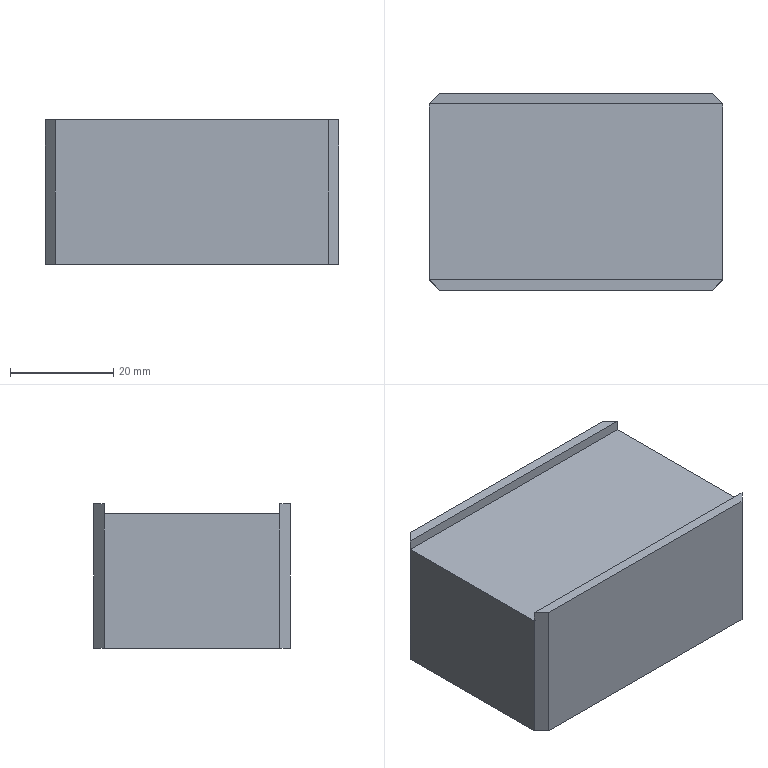Part | SolidWorks | features Chamfer 1, Cut 1, Extrusion 1 | 1 solid | 14 faces | box 56.8 x 38 x 28 mm | volume 56349 mm3 | plane 14
STEP:
#1=CARTESIAN_POINT('',(-26.4,19.,14.));
#2=VERTEX_POINT('',#1);
#3=CARTESIAN_POINT('',(-28.4,17.,14.));
#4=VERTEX_POINT('',#3);
#5=CARTESIAN_POINT('',(-28.4,17.,14.));
#6=DIRECTION('',(-0.7071,-0.7071,0.));
#7=VECTOR('',#6,1000.);
#8=LINE('',#5,#7);
#9=EDGE_CURVE('',#2,#4,#8,.T.);
#10=ORIENTED_EDGE('',*,*,#9,.T.);
#11=CARTESIAN_POINT('',(28.4,17.,14.));
#12=VERTEX_POINT('',#11);
#13=CARTESIAN_POINT('',(-28.4,17.,14.));
#14=DIRECTION('',(1.,0.,0.));
#15=VECTOR('',#14,1000.);
#16=LINE('',#13,#15);
#17=EDGE_CURVE('',#4,#12,#16,.T.);
#18=ORIENTED_EDGE('',*,*,#17,.T.);
#19=CARTESIAN_POINT('',(26.4,19.,14.));
#20=VERTEX_POINT('',#19);
#21=CARTESIAN_POINT('',(26.4,19.,14.));
#22=DIRECTION('',(-0.7071,0.7071,0.));
#23=VECTOR('',#22,1000.);
#24=LINE('',#21,#23);
#25=EDGE_CURVE('',#12,#20,#24,.T.);
#26=ORIENTED_EDGE('',*,*,#25,.T.);
#27=CARTESIAN_POINT('',(-28.4,19.,14.));
#28=DIRECTION('',(-1.,0.,0.));
#29=VECTOR('',#28,1000.);
#30=LINE('',#27,#29);
#31=EDGE_CURVE('',#20,#2,#30,.T.);
#32=ORIENTED_EDGE('',*,*,#31,.T.);
#33=EDGE_LOOP('',(#10,#18,#26,#32));
#34=FACE_OUTER_BOUND('',#33,.T.);
#35=CARTESIAN_POINT('',(0.,0.,14.));
#36=DIRECTION('',(0.,0.,-1.));
#37=DIRECTION('',(-1.,0.,0.));
#38=AXIS2_PLACEMENT_3D('',#35,#36,#37);
#39=PLANE('',#38);
#40=ADVANCED_FACE('',(#34),#39,.F.);
#41=CARTESIAN_POINT('',(28.4,17.,-14.));
#42=VERTEX_POINT('',#41);
#43=CARTESIAN_POINT('',(28.4,17.,12.));
#44=VERTEX_POINT('',#43);
#45=CARTESIAN_POINT('',(28.4,17.,14.));
#46=DIRECTION('',(0.,0.,1.));
#47=VECTOR('',#46,1000.);
#48=LINE('',#45,#47);
#49=EDGE_CURVE('',#42,#44,#48,.T.);
#50=ORIENTED_EDGE('',*,*,#49,.T.);
#51=CARTESIAN_POINT('',(28.4,-17.,12.));
#52=VERTEX_POINT('',#51);
#53=CARTESIAN_POINT('',(28.4,17.,12.));
#54=DIRECTION('',(0.,1.,0.));
#55=VECTOR('',#54,1000.);
#56=LINE('',#53,#55);
#57=EDGE_CURVE('',#52,#44,#56,.T.);
#58=ORIENTED_EDGE('',*,*,#57,.F.);
#59=CARTESIAN_POINT('',(28.4,-17.,-14.));
#60=VERTEX_POINT('',#59);
#61=CARTESIAN_POINT('',(28.4,-17.,14.));
#62=DIRECTION('',(0.,0.,-1.));
#63=VECTOR('',#62,1000.);
#64=LINE('',#61,#63);
#65=EDGE_CURVE('',#52,#60,#64,.T.);
#66=ORIENTED_EDGE('',*,*,#65,.T.);
#67=CARTESIAN_POINT('',(28.4,-19.,-14.));
#68=DIRECTION('',(0.,1.,0.));
#69=VECTOR('',#68,1000.);
#70=LINE('',#67,#69);
#71=EDGE_CURVE('',#60,#42,#70,.T.);
#72=ORIENTED_EDGE('',*,*,#71,.T.);
#73=EDGE_LOOP('',(#50,#58,#66,#72));
#74=FACE_OUTER_BOUND('',#73,.T.);
#75=CARTESIAN_POINT('',(28.4,-19.,14.));
#76=DIRECTION('',(-1.,0.,0.));
#77=DIRECTION('',(0.,0.,1.));
#78=AXIS2_PLACEMENT_3D('',#75,#76,#77);
#79=PLANE('',#78);
#80=ADVANCED_FACE('',(#74),#79,.F.);
#81=CARTESIAN_POINT('',(26.4,19.,-14.));
#82=VERTEX_POINT('',#81);
#83=CARTESIAN_POINT('',(-26.4,19.,-14.));
#84=VERTEX_POINT('',#83);
#85=CARTESIAN_POINT('',(-28.4,19.,-14.));
#86=DIRECTION('',(-1.,0.,0.));
#87=VECTOR('',#86,1000.);
#88=LINE('',#85,#87);
#89=EDGE_CURVE('',#82,#84,#88,.T.);
#90=ORIENTED_EDGE('',*,*,#89,.T.);
#91=CARTESIAN_POINT('',(-26.4,19.,14.));
#92=DIRECTION('',(0.,0.,1.));
#93=VECTOR('',#92,1000.);
#94=LINE('',#91,#93);
#95=EDGE_CURVE('',#84,#2,#94,.T.);
#96=ORIENTED_EDGE('',*,*,#95,.T.);
#97=ORIENTED_EDGE('',*,*,#31,.F.);
#98=CARTESIAN_POINT('',(26.4,19.,14.));
#99=DIRECTION('',(0.,0.,-1.));
#100=VECTOR('',#99,1000.);
#101=LINE('',#98,#100);
#102=EDGE_CURVE('',#20,#82,#101,.T.);
#103=ORIENTED_EDGE('',*,*,#102,.T.);
#104=EDGE_LOOP('',(#90,#96,#97,#103));
#105=FACE_OUTER_BOUND('',#104,.T.);
#106=CARTESIAN_POINT('',(-28.4,19.,14.));
#107=DIRECTION('',(0.,-1.,0.));
#108=DIRECTION('',(0.,0.,-1.));
#109=AXIS2_PLACEMENT_3D('',#106,#107,#108);
#110=PLANE('',#109);
#111=ADVANCED_FACE('',(#105),#110,.F.);
#112=CARTESIAN_POINT('',(-28.4,-17.,-14.));
#113=VERTEX_POINT('',#112);
#114=CARTESIAN_POINT('',(-28.4,-17.,12.));
#115=VERTEX_POINT('',#114);
#116=CARTESIAN_POINT('',(-28.4,-17.,14.));
#117=DIRECTION('',(0.,0.,1.));
#118=VECTOR('',#117,1000.);
#119=LINE('',#116,#118);
#120=EDGE_CURVE('',#113,#115,#119,.T.);
#121=ORIENTED_EDGE('',*,*,#120,.T.);
#122=CARTESIAN_POINT('',(-28.4,17.,12.));
#123=VERTEX_POINT('',#122);
#124=CARTESIAN_POINT('',(-28.4,17.,12.));
#125=DIRECTION('',(0.,1.,0.));
#126=VECTOR('',#125,1000.);
#127=LINE('',#124,#126);
#128=EDGE_CURVE('',#115,#123,#127,.T.);
#129=ORIENTED_EDGE('',*,*,#128,.T.);
#130=CARTESIAN_POINT('',(-28.4,17.,-14.));
#131=VERTEX_POINT('',#130);
#132=CARTESIAN_POINT('',(-28.4,17.,14.));
#133=DIRECTION('',(0.,0.,-1.));
#134=VECTOR('',#133,1000.);
#135=LINE('',#132,#134);
#136=EDGE_CURVE('',#123,#131,#135,.T.);
#137=ORIENTED_EDGE('',*,*,#136,.T.);
#138=CARTESIAN_POINT('',(-28.4,-19.,-14.));
#139=DIRECTION('',(0.,-1.,0.));
#140=VECTOR('',#139,1000.);
#141=LINE('',#138,#140);
#142=EDGE_CURVE('',#131,#113,#141,.T.);
#143=ORIENTED_EDGE('',*,*,#142,.T.);
#144=EDGE_LOOP('',(#121,#129,#137,#143));
#145=FACE_OUTER_BOUND('',#144,.T.);
#146=CARTESIAN_POINT('',(-28.4,-19.,14.));
#147=DIRECTION('',(1.,0.,0.));
#148=DIRECTION('',(0.,0.,-1.));
#149=AXIS2_PLACEMENT_3D('',#146,#147,#148);
#150=PLANE('',#149);
#151=ADVANCED_FACE('',(#145),#150,.F.);
#152=CARTESIAN_POINT('',(-26.4,-19.,-14.));
#153=VERTEX_POINT('',#152);
#154=CARTESIAN_POINT('',(26.4,-19.,-14.));
#155=VERTEX_POINT('',#154);
#156=CARTESIAN_POINT('',(-28.4,-19.,-14.));
#157=DIRECTION('',(1.,0.,0.));
#158=VECTOR('',#157,1000.);
#159=LINE('',#156,#158);
#160=EDGE_CURVE('',#153,#155,#159,.T.);
#161=ORIENTED_EDGE('',*,*,#160,.T.);
#162=CARTESIAN_POINT('',(26.4,-19.,14.));
#163=VERTEX_POINT('',#162);
#164=CARTESIAN_POINT('',(26.4,-19.,14.));
#165=DIRECTION('',(0.,0.,1.));
#166=VECTOR('',#165,1000.);
#167=LINE('',#164,#166);
#168=EDGE_CURVE('',#155,#163,#167,.T.);
#169=ORIENTED_EDGE('',*,*,#168,.T.);
#170=CARTESIAN_POINT('',(-26.4,-19.,14.));
#171=VERTEX_POINT('',#170);
#172=CARTESIAN_POINT('',(-28.4,-19.,14.));
#173=DIRECTION('',(1.,0.,0.));
#174=VECTOR('',#173,1000.);
#175=LINE('',#172,#174);
#176=EDGE_CURVE('',#171,#163,#175,.T.);
#177=ORIENTED_EDGE('',*,*,#176,.F.);
#178=CARTESIAN_POINT('',(-26.4,-19.,14.));
#179=DIRECTION('',(0.,0.,-1.));
#180=VECTOR('',#179,1000.);
#181=LINE('',#178,#180);
#182=EDGE_CURVE('',#171,#153,#181,.T.);
#183=ORIENTED_EDGE('',*,*,#182,.T.);
#184=EDGE_LOOP('',(#161,#169,#177,#183));
#185=FACE_OUTER_BOUND('',#184,.T.);
#186=CARTESIAN_POINT('',(-28.4,-19.,14.));
#187=DIRECTION('',(0.,1.,0.));
#188=DIRECTION('',(0.,0.,1.));
#189=AXIS2_PLACEMENT_3D('',#186,#187,#188);
#190=PLANE('',#189);
#191=ADVANCED_FACE('',(#185),#190,.F.);
#192=CARTESIAN_POINT('',(28.4,-17.,14.));
#193=VERTEX_POINT('',#192);
#194=CARTESIAN_POINT('',(28.4,-17.,14.));
#195=DIRECTION('',(0.7071,0.7071,0.));
#196=VECTOR('',#195,1000.);
#197=LINE('',#194,#196);
#198=EDGE_CURVE('',#163,#193,#197,.T.);
#199=ORIENTED_EDGE('',*,*,#198,.T.);
#200=CARTESIAN_POINT('',(-28.4,-17.,14.));
#201=VERTEX_POINT('',#200);
#202=CARTESIAN_POINT('',(-28.4,-17.,14.));
#203=DIRECTION('',(1.,0.,0.));
#204=VECTOR('',#203,1000.);
#205=LINE('',#202,#204);
#206=EDGE_CURVE('',#201,#193,#205,.T.);
#207=ORIENTED_EDGE('',*,*,#206,.F.);
#208=CARTESIAN_POINT('',(-26.4,-19.,14.));
#209=DIRECTION('',(0.7071,-0.7071,0.));
#210=VECTOR('',#209,1000.);
#211=LINE('',#208,#210);
#212=EDGE_CURVE('',#201,#171,#211,.T.);
#213=ORIENTED_EDGE('',*,*,#212,.T.);
#214=ORIENTED_EDGE('',*,*,#176,.T.);
#215=EDGE_LOOP('',(#199,#207,#213,#214));
#216=FACE_OUTER_BOUND('',#215,.T.);
#217=CARTESIAN_POINT('',(0.,0.,14.));
#218=DIRECTION('',(0.,0.,-1.));
#219=DIRECTION('',(-1.,0.,0.));
#220=AXIS2_PLACEMENT_3D('',#217,#218,#219);
#221=PLANE('',#220);
#222=ADVANCED_FACE('',(#216),#221,.F.);
#223=ORIENTED_EDGE('',*,*,#71,.F.);
#224=CARTESIAN_POINT('',(22.7,-22.7,-14.));
#225=DIRECTION('',(-0.7071,-0.7071,0.));
#226=VECTOR('',#225,1000.);
#227=LINE('',#224,#226);
#228=EDGE_CURVE('',#60,#155,#227,.T.);
#229=ORIENTED_EDGE('',*,*,#228,.T.);
#230=ORIENTED_EDGE('',*,*,#160,.F.);
#231=CARTESIAN_POINT('',(-22.7,-22.7,-14.));
#232=DIRECTION('',(-0.7071,0.7071,0.));
#233=VECTOR('',#232,1000.);
#234=LINE('',#231,#233);
#235=EDGE_CURVE('',#153,#113,#234,.T.);
#236=ORIENTED_EDGE('',*,*,#235,.T.);
#237=ORIENTED_EDGE('',*,*,#142,.F.);
#238=CARTESIAN_POINT('',(-22.7,22.7,-14.));
#239=DIRECTION('',(0.7071,0.7071,0.));
#240=VECTOR('',#239,1000.);
#241=LINE('',#238,#240);
#242=EDGE_CURVE('',#131,#84,#241,.T.);
#243=ORIENTED_EDGE('',*,*,#242,.T.);
#244=ORIENTED_EDGE('',*,*,#89,.F.);
#245=CARTESIAN_POINT('',(22.7,22.7,-14.));
#246=DIRECTION('',(0.7071,-0.7071,0.));
#247=VECTOR('',#246,1000.);
#248=LINE('',#245,#247);
#249=EDGE_CURVE('',#82,#42,#248,.T.);
#250=ORIENTED_EDGE('',*,*,#249,.T.);
#251=EDGE_LOOP('',(#223,#229,#230,#236,#237,#243,#244,#250));
#252=FACE_OUTER_BOUND('',#251,.T.);
#253=CARTESIAN_POINT('',(0.,0.,-14.));
#254=DIRECTION('',(0.,0.,-1.));
#255=DIRECTION('',(-1.,0.,0.));
#256=AXIS2_PLACEMENT_3D('',#253,#254,#255);
#257=PLANE('',#256);
#258=ADVANCED_FACE('',(#252),#257,.T.);
#259=ORIENTED_EDGE('',*,*,#198,.F.);
#260=ORIENTED_EDGE('',*,*,#168,.F.);
#261=ORIENTED_EDGE('',*,*,#228,.F.);
#262=ORIENTED_EDGE('',*,*,#65,.F.);
#263=CARTESIAN_POINT('',(28.4,-17.,14.));
#264=DIRECTION('',(0.,0.,-1.));
#265=VECTOR('',#264,1000.);
#266=LINE('',#263,#265);
#267=EDGE_CURVE('',#193,#52,#266,.T.);
#268=ORIENTED_EDGE('',*,*,#267,.F.);
#269=EDGE_LOOP('',(#259,#260,#261,#262,#268));
#270=FACE_OUTER_BOUND('',#269,.T.);
#271=CARTESIAN_POINT('',(28.4,-17.,14.));
#272=DIRECTION('',(-0.7071,0.7071,0.));
#273=DIRECTION('',(0.,0.,-1.));
#274=AXIS2_PLACEMENT_3D('',#271,#272,#273);
#275=PLANE('',#274);
#276=ADVANCED_FACE('',(#270),#275,.F.);
#277=ORIENTED_EDGE('',*,*,#212,.F.);
#278=CARTESIAN_POINT('',(-28.4,-17.,14.));
#279=DIRECTION('',(0.,0.,-1.));
#280=VECTOR('',#279,1000.);
#281=LINE('',#278,#280);
#282=EDGE_CURVE('',#201,#115,#281,.T.);
#283=ORIENTED_EDGE('',*,*,#282,.T.);
#284=ORIENTED_EDGE('',*,*,#120,.F.);
#285=ORIENTED_EDGE('',*,*,#235,.F.);
#286=ORIENTED_EDGE('',*,*,#182,.F.);
#287=EDGE_LOOP('',(#277,#283,#284,#285,#286));
#288=FACE_OUTER_BOUND('',#287,.T.);
#289=CARTESIAN_POINT('',(-26.4,-19.,14.));
#290=DIRECTION('',(0.7071,0.7071,0.));
#291=DIRECTION('',(0.,0.,-1.));
#292=AXIS2_PLACEMENT_3D('',#289,#290,#291);
#293=PLANE('',#292);
#294=ADVANCED_FACE('',(#288),#293,.F.);
#295=ORIENTED_EDGE('',*,*,#9,.F.);
#296=ORIENTED_EDGE('',*,*,#95,.F.);
#297=ORIENTED_EDGE('',*,*,#242,.F.);
#298=ORIENTED_EDGE('',*,*,#136,.F.);
#299=CARTESIAN_POINT('',(-28.4,17.,14.));
#300=DIRECTION('',(0.,0.,-1.));
#301=VECTOR('',#300,1000.);
#302=LINE('',#299,#301);
#303=EDGE_CURVE('',#4,#123,#302,.T.);
#304=ORIENTED_EDGE('',*,*,#303,.F.);
#305=EDGE_LOOP('',(#295,#296,#297,#298,#304));
#306=FACE_OUTER_BOUND('',#305,.T.);
#307=CARTESIAN_POINT('',(-28.4,17.,14.));
#308=DIRECTION('',(0.7071,-0.7071,0.));
#309=DIRECTION('',(0.,0.,-1.));
#310=AXIS2_PLACEMENT_3D('',#307,#308,#309);
#311=PLANE('',#310);
#312=ADVANCED_FACE('',(#306),#311,.F.);
#313=ORIENTED_EDGE('',*,*,#25,.F.);
#314=CARTESIAN_POINT('',(28.4,17.,14.));
#315=DIRECTION('',(0.,0.,1.));
#316=VECTOR('',#315,1000.);
#317=LINE('',#314,#316);
#318=EDGE_CURVE('',#44,#12,#317,.T.);
#319=ORIENTED_EDGE('',*,*,#318,.F.);
#320=ORIENTED_EDGE('',*,*,#49,.F.);
#321=ORIENTED_EDGE('',*,*,#249,.F.);
#322=ORIENTED_EDGE('',*,*,#102,.F.);
#323=EDGE_LOOP('',(#313,#319,#320,#321,#322));
#324=FACE_OUTER_BOUND('',#323,.T.);
#325=CARTESIAN_POINT('',(26.4,19.,14.));
#326=DIRECTION('',(-0.7071,-0.7071,0.));
#327=DIRECTION('',(0.,0.,-1.));
#328=AXIS2_PLACEMENT_3D('',#325,#326,#327);
#329=PLANE('',#328);
#330=ADVANCED_FACE('',(#324),#329,.F.);
#331=ORIENTED_EDGE('',*,*,#318,.T.);
#332=ORIENTED_EDGE('',*,*,#17,.F.);
#333=ORIENTED_EDGE('',*,*,#303,.T.);
#334=CARTESIAN_POINT('',(-28.4,17.,12.));
#335=DIRECTION('',(1.,0.,0.));
#336=VECTOR('',#335,1000.);
#337=LINE('',#334,#336);
#338=EDGE_CURVE('',#123,#44,#337,.T.);
#339=ORIENTED_EDGE('',*,*,#338,.T.);
#340=EDGE_LOOP('',(#331,#332,#333,#339));
#341=FACE_OUTER_BOUND('',#340,.T.);
#342=CARTESIAN_POINT('',(-28.4,17.,14.));
#343=DIRECTION('',(0.,1.,0.));
#344=DIRECTION('',(0.,0.,1.));
#345=AXIS2_PLACEMENT_3D('',#342,#343,#344);
#346=PLANE('',#345);
#347=ADVANCED_FACE('',(#341),#346,.F.);
#348=ORIENTED_EDGE('',*,*,#57,.T.);
#349=ORIENTED_EDGE('',*,*,#338,.F.);
#350=ORIENTED_EDGE('',*,*,#128,.F.);
#351=CARTESIAN_POINT('',(-28.4,-17.,12.));
#352=DIRECTION('',(1.,0.,0.));
#353=VECTOR('',#352,1000.);
#354=LINE('',#351,#353);
#355=EDGE_CURVE('',#115,#52,#354,.T.);
#356=ORIENTED_EDGE('',*,*,#355,.T.);
#357=EDGE_LOOP('',(#348,#349,#350,#356));
#358=FACE_OUTER_BOUND('',#357,.T.);
#359=CARTESIAN_POINT('',(-28.4,17.,12.));
#360=DIRECTION('',(0.,0.,-1.));
#361=DIRECTION('',(-1.,0.,0.));
#362=AXIS2_PLACEMENT_3D('',#359,#360,#361);
#363=PLANE('',#362);
#364=ADVANCED_FACE('',(#358),#363,.F.);
#365=ORIENTED_EDGE('',*,*,#267,.T.);
#366=ORIENTED_EDGE('',*,*,#355,.F.);
#367=ORIENTED_EDGE('',*,*,#282,.F.);
#368=ORIENTED_EDGE('',*,*,#206,.T.);
#369=EDGE_LOOP('',(#365,#366,#367,#368));
#370=FACE_OUTER_BOUND('',#369,.T.);
#371=CARTESIAN_POINT('',(-28.4,-17.,14.));
#372=DIRECTION('',(0.,-1.,0.));
#373=DIRECTION('',(0.,0.,-1.));
#374=AXIS2_PLACEMENT_3D('',#371,#372,#373);
#375=PLANE('',#374);
#376=ADVANCED_FACE('',(#370),#375,.F.);
#377=CLOSED_SHELL('',(#40,#80,#111,#151,#191,#222,#258,#276,#294,#312,#330,#347,#364,#376));
#378=MANIFOLD_SOLID_BREP('',#377);
#379=CARTESIAN_POINT('',(0.,0.,0.));
#380=DIRECTION('',(0.,0.,1.));
#381=DIRECTION('',(1.,0.,0.));
#382=AXIS2_PLACEMENT_3D('',#379,#380,#381);
#383=(LENGTH_UNIT()NAMED_UNIT(*)SI_UNIT(.MILLI.,.METRE.));
#384=UNCERTAINTY_MEASURE_WITH_UNIT(LENGTH_MEASURE(0.00001),#383,'','');
#385=(NAMED_UNIT(*)PLANE_ANGLE_UNIT()SI_UNIT($,.RADIAN.));
#386=(NAMED_UNIT(*)SI_UNIT($,.STERADIAN.)SOLID_ANGLE_UNIT());
#387=(GEOMETRIC_REPRESENTATION_CONTEXT(3)GLOBAL_UNCERTAINTY_ASSIGNED_CONTEXT((#384))GLOBAL_UNIT_ASSIGNED_CONTEXT((#383,#385,#386))REPRESENTATION_CONTEXT('',''));
#388=ADVANCED_BREP_SHAPE_REPRESENTATION('',(#378,#382),#387);